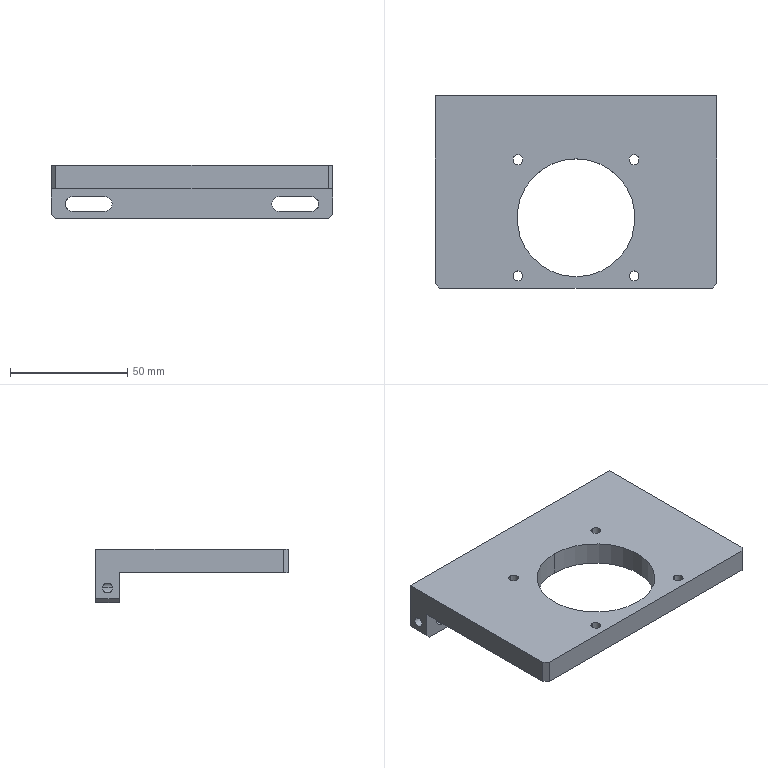Part | 1 solid | 36 faces | box 120 x 82 x 22.8 mm | volume 90820 mm3 | cylinder 20 | plane 16 | commonest cylinder face diameters 4.2 x12 6.3 x6 50.2 x2
STEP:
#1=CARTESIAN_POINT('',(-24.749,-37.849,0.));
#2=VERTEX_POINT('',#1);
#3=CARTESIAN_POINT('',(-24.749,-33.649,0.));
#4=VERTEX_POINT('',#3);
#5=CARTESIAN_POINT('',(-24.749,-35.749,0.));
#6=DIRECTION('',(0.,0.,-1.));
#7=DIRECTION('',(0.,1.,0.));
#8=AXIS2_PLACEMENT_3D('',#5,#6,#7);
#9=CIRCLE('',#8,2.1);
#10=EDGE_CURVE('',#2,#4,#9,.T.);
#11=ORIENTED_EDGE('',*,*,#10,.F.);
#12=CARTESIAN_POINT('',(-24.749,-37.849,-10.));
#13=VERTEX_POINT('',#12);
#14=CARTESIAN_POINT('',(-24.749,-37.849,-10.));
#15=DIRECTION('',(0.,0.,-1.));
#16=VECTOR('',#15,1000.);
#17=LINE('',#14,#16);
#18=EDGE_CURVE('',#13,#2,#17,.F.);
#19=ORIENTED_EDGE('',*,*,#18,.F.);
#20=CARTESIAN_POINT('',(-24.749,-33.649,-10.));
#21=VERTEX_POINT('',#20);
#22=CARTESIAN_POINT('',(-24.749,-35.749,-10.));
#23=DIRECTION('',(0.,0.,-1.));
#24=DIRECTION('',(0.,1.,0.));
#25=AXIS2_PLACEMENT_3D('',#22,#23,#24);
#26=CIRCLE('',#25,2.1);
#27=EDGE_CURVE('',#13,#21,#26,.T.);
#28=ORIENTED_EDGE('',*,*,#27,.T.);
#29=CARTESIAN_POINT('',(-24.749,-33.649,-10.));
#30=DIRECTION('',(0.,0.,-1.));
#31=VECTOR('',#30,1000.);
#32=LINE('',#29,#31);
#33=EDGE_CURVE('',#21,#4,#32,.F.);
#34=ORIENTED_EDGE('',*,*,#33,.T.);
#35=EDGE_LOOP('',(#11,#19,#28,#34));
#36=FACE_BOUND('',#35,.T.);
#37=CARTESIAN_POINT('',(-24.749,-35.749,-10.));
#38=DIRECTION('',(0.,0.,-1.));
#39=DIRECTION('',(0.,-1.,0.));
#40=AXIS2_PLACEMENT_3D('',#37,#38,#39);
#41=CYLINDRICAL_SURFACE('',#40,2.1);
#42=ADVANCED_FACE('',(#36),#41,.F.);
#43=CARTESIAN_POINT('',(24.749,-37.849,0.));
#44=VERTEX_POINT('',#43);
#45=CARTESIAN_POINT('',(24.749,-33.649,0.));
#46=VERTEX_POINT('',#45);
#47=CARTESIAN_POINT('',(24.749,-35.749,0.));
#48=DIRECTION('',(0.,0.,-1.));
#49=DIRECTION('',(0.,1.,0.));
#50=AXIS2_PLACEMENT_3D('',#47,#48,#49);
#51=CIRCLE('',#50,2.1);
#52=EDGE_CURVE('',#44,#46,#51,.T.);
#53=ORIENTED_EDGE('',*,*,#52,.F.);
#54=CARTESIAN_POINT('',(24.749,-37.849,-10.));
#55=VERTEX_POINT('',#54);
#56=CARTESIAN_POINT('',(24.749,-37.849,-10.));
#57=DIRECTION('',(0.,0.,-1.));
#58=VECTOR('',#57,1000.);
#59=LINE('',#56,#58);
#60=EDGE_CURVE('',#55,#44,#59,.F.);
#61=ORIENTED_EDGE('',*,*,#60,.F.);
#62=CARTESIAN_POINT('',(24.749,-33.649,-10.));
#63=VERTEX_POINT('',#62);
#64=CARTESIAN_POINT('',(24.749,-35.749,-10.));
#65=DIRECTION('',(0.,0.,-1.));
#66=DIRECTION('',(0.,1.,0.));
#67=AXIS2_PLACEMENT_3D('',#64,#65,#66);
#68=CIRCLE('',#67,2.1);
#69=EDGE_CURVE('',#55,#63,#68,.T.);
#70=ORIENTED_EDGE('',*,*,#69,.T.);
#71=CARTESIAN_POINT('',(24.749,-33.649,-10.));
#72=DIRECTION('',(0.,0.,-1.));
#73=VECTOR('',#72,1000.);
#74=LINE('',#71,#73);
#75=EDGE_CURVE('',#63,#46,#74,.F.);
#76=ORIENTED_EDGE('',*,*,#75,.T.);
#77=EDGE_LOOP('',(#53,#61,#70,#76));
#78=FACE_BOUND('',#77,.T.);
#79=CARTESIAN_POINT('',(24.749,-35.749,-10.));
#80=DIRECTION('',(0.,0.,-1.));
#81=DIRECTION('',(0.,-1.,0.));
#82=AXIS2_PLACEMENT_3D('',#79,#80,#81);
#83=CYLINDRICAL_SURFACE('',#82,2.1);
#84=ADVANCED_FACE('',(#78),#83,.F.);
#85=CARTESIAN_POINT('',(-24.749,11.649,0.));
#86=VERTEX_POINT('',#85);
#87=CARTESIAN_POINT('',(-24.749,15.849,0.));
#88=VERTEX_POINT('',#87);
#89=CARTESIAN_POINT('',(-24.749,13.749,0.));
#90=DIRECTION('',(0.,0.,-1.));
#91=DIRECTION('',(0.,1.,0.));
#92=AXIS2_PLACEMENT_3D('',#89,#90,#91);
#93=CIRCLE('',#92,2.1);
#94=EDGE_CURVE('',#86,#88,#93,.T.);
#95=ORIENTED_EDGE('',*,*,#94,.F.);
#96=CARTESIAN_POINT('',(-24.749,11.649,-10.));
#97=VERTEX_POINT('',#96);
#98=CARTESIAN_POINT('',(-24.749,11.649,-10.));
#99=DIRECTION('',(0.,0.,-1.));
#100=VECTOR('',#99,1000.);
#101=LINE('',#98,#100);
#102=EDGE_CURVE('',#97,#86,#101,.F.);
#103=ORIENTED_EDGE('',*,*,#102,.F.);
#104=CARTESIAN_POINT('',(-24.749,15.849,-10.));
#105=VERTEX_POINT('',#104);
#106=CARTESIAN_POINT('',(-24.749,13.749,-10.));
#107=DIRECTION('',(0.,0.,-1.));
#108=DIRECTION('',(0.,1.,0.));
#109=AXIS2_PLACEMENT_3D('',#106,#107,#108);
#110=CIRCLE('',#109,2.1);
#111=EDGE_CURVE('',#97,#105,#110,.T.);
#112=ORIENTED_EDGE('',*,*,#111,.T.);
#113=CARTESIAN_POINT('',(-24.749,15.849,-10.));
#114=DIRECTION('',(0.,0.,-1.));
#115=VECTOR('',#114,1000.);
#116=LINE('',#113,#115);
#117=EDGE_CURVE('',#105,#88,#116,.F.);
#118=ORIENTED_EDGE('',*,*,#117,.T.);
#119=EDGE_LOOP('',(#95,#103,#112,#118));
#120=FACE_BOUND('',#119,.T.);
#121=CARTESIAN_POINT('',(-24.749,13.749,-10.));
#122=DIRECTION('',(0.,0.,-1.));
#123=DIRECTION('',(0.,-1.,0.));
#124=AXIS2_PLACEMENT_3D('',#121,#122,#123);
#125=CYLINDRICAL_SURFACE('',#124,2.1);
#126=ADVANCED_FACE('',(#120),#125,.F.);
#127=CARTESIAN_POINT('',(24.749,11.649,0.));
#128=VERTEX_POINT('',#127);
#129=CARTESIAN_POINT('',(24.749,15.849,0.));
#130=VERTEX_POINT('',#129);
#131=CARTESIAN_POINT('',(24.749,13.749,0.));
#132=DIRECTION('',(0.,0.,-1.));
#133=DIRECTION('',(0.,1.,0.));
#134=AXIS2_PLACEMENT_3D('',#131,#132,#133);
#135=CIRCLE('',#134,2.1);
#136=EDGE_CURVE('',#128,#130,#135,.T.);
#137=ORIENTED_EDGE('',*,*,#136,.F.);
#138=CARTESIAN_POINT('',(24.749,11.649,-10.));
#139=VERTEX_POINT('',#138);
#140=CARTESIAN_POINT('',(24.749,11.649,-10.));
#141=DIRECTION('',(0.,0.,-1.));
#142=VECTOR('',#141,1000.);
#143=LINE('',#140,#142);
#144=EDGE_CURVE('',#139,#128,#143,.F.);
#145=ORIENTED_EDGE('',*,*,#144,.F.);
#146=CARTESIAN_POINT('',(24.749,15.849,-10.));
#147=VERTEX_POINT('',#146);
#148=CARTESIAN_POINT('',(24.749,13.749,-10.));
#149=DIRECTION('',(0.,0.,-1.));
#150=DIRECTION('',(0.,1.,0.));
#151=AXIS2_PLACEMENT_3D('',#148,#149,#150);
#152=CIRCLE('',#151,2.1);
#153=EDGE_CURVE('',#139,#147,#152,.T.);
#154=ORIENTED_EDGE('',*,*,#153,.T.);
#155=CARTESIAN_POINT('',(24.749,15.849,-10.));
#156=DIRECTION('',(0.,0.,-1.));
#157=VECTOR('',#156,1000.);
#158=LINE('',#155,#157);
#159=EDGE_CURVE('',#147,#130,#158,.F.);
#160=ORIENTED_EDGE('',*,*,#159,.T.);
#161=EDGE_LOOP('',(#137,#145,#154,#160));
#162=FACE_BOUND('',#161,.T.);
#163=CARTESIAN_POINT('',(24.749,13.749,-10.));
#164=DIRECTION('',(0.,0.,-1.));
#165=DIRECTION('',(0.,-1.,0.));
#166=AXIS2_PLACEMENT_3D('',#163,#164,#165);
#167=CYLINDRICAL_SURFACE('',#166,2.1);
#168=ADVANCED_FACE('',(#162),#167,.F.);
#169=CARTESIAN_POINT('',(0.,14.1,-10.));
#170=VERTEX_POINT('',#169);
#171=CARTESIAN_POINT('',(0.,-36.1,-10.));
#172=VERTEX_POINT('',#171);
#173=CARTESIAN_POINT('',(0.,-11.,-10.));
#174=DIRECTION('',(0.,0.,1.));
#175=DIRECTION('',(-1.,0.,0.));
#176=AXIS2_PLACEMENT_3D('',#173,#174,#175);
#177=CIRCLE('',#176,25.1);
#178=EDGE_CURVE('',#170,#172,#177,.T.);
#179=ORIENTED_EDGE('',*,*,#178,.F.);
#180=CARTESIAN_POINT('',(0.,14.1,0.));
#181=VERTEX_POINT('',#180);
#182=CARTESIAN_POINT('',(0.,14.1,0.));
#183=DIRECTION('',(0.,0.,1.));
#184=VECTOR('',#183,1000.);
#185=LINE('',#182,#184);
#186=EDGE_CURVE('',#181,#170,#185,.F.);
#187=ORIENTED_EDGE('',*,*,#186,.F.);
#188=CARTESIAN_POINT('',(0.,-36.1,0.));
#189=VERTEX_POINT('',#188);
#190=CARTESIAN_POINT('',(0.,-11.,0.));
#191=DIRECTION('',(0.,0.,1.));
#192=DIRECTION('',(0.,-1.,0.));
#193=AXIS2_PLACEMENT_3D('',#190,#191,#192);
#194=CIRCLE('',#193,25.1);
#195=EDGE_CURVE('',#181,#189,#194,.T.);
#196=ORIENTED_EDGE('',*,*,#195,.T.);
#197=CARTESIAN_POINT('',(0.,-36.1,0.));
#198=DIRECTION('',(0.,0.,1.));
#199=VECTOR('',#198,1000.);
#200=LINE('',#197,#199);
#201=EDGE_CURVE('',#189,#172,#200,.F.);
#202=ORIENTED_EDGE('',*,*,#201,.T.);
#203=EDGE_LOOP('',(#179,#187,#196,#202));
#204=FACE_BOUND('',#203,.T.);
#205=CARTESIAN_POINT('',(0.,-11.,0.));
#206=DIRECTION('',(0.,0.,1.));
#207=DIRECTION('',(0.,1.,0.));
#208=AXIS2_PLACEMENT_3D('',#205,#206,#207);
#209=CYLINDRICAL_SURFACE('',#208,25.1);
#210=ADVANCED_FACE('',(#204),#209,.F.);
#211=CARTESIAN_POINT('',(54.,33.9,-16.5));
#212=VERTEX_POINT('',#211);
#213=CARTESIAN_POINT('',(54.,38.1,-16.5));
#214=VERTEX_POINT('',#213);
#215=CARTESIAN_POINT('',(54.,33.9,-16.5));
#216=CARTESIAN_POINT('',(54.,33.9,-17.075));
#217=CARTESIAN_POINT('',(53.653,34.362,-18.14));
#218=CARTESIAN_POINT('',(52.971,35.995,-18.829));
#219=CARTESIAN_POINT('',(53.651,37.638,-18.143));
#220=CARTESIAN_POINT('',(54.,38.1,-17.075));
#221=CARTESIAN_POINT('',(54.,38.1,-16.5));
#222=B_SPLINE_CURVE_WITH_KNOTS('',3,(#215,#216,#217,#218,#219,#220,#221),.UNSPECIFIED.,.F.,.F.,(4,1,1,1,4),(0.,0.001696,0.003392,0.005088,0.006784),.UNSPECIFIED.);
#223=EDGE_CURVE('',#212,#214,#222,.T.);
#224=ORIENTED_EDGE('',*,*,#223,.F.);
#225=CARTESIAN_POINT('',(60.,33.9,-16.5));
#226=VERTEX_POINT('',#225);
#227=CARTESIAN_POINT('',(60.,33.9,-16.5));
#228=DIRECTION('',(1.,0.,0.));
#229=VECTOR('',#228,1000.);
#230=LINE('',#227,#229);
#231=EDGE_CURVE('',#226,#212,#230,.F.);
#232=ORIENTED_EDGE('',*,*,#231,.F.);
#233=CARTESIAN_POINT('',(60.,38.1,-16.5));
#234=VERTEX_POINT('',#233);
#235=CARTESIAN_POINT('',(60.,36.,-16.5));
#236=DIRECTION('',(1.,0.,0.));
#237=DIRECTION('',(0.,1.,0.));
#238=AXIS2_PLACEMENT_3D('',#235,#236,#237);
#239=CIRCLE('',#238,2.1);
#240=EDGE_CURVE('',#226,#234,#239,.T.);
#241=ORIENTED_EDGE('',*,*,#240,.T.);
#242=CARTESIAN_POINT('',(60.,38.1,-16.5));
#243=DIRECTION('',(1.,0.,0.));
#244=VECTOR('',#243,1000.);
#245=LINE('',#242,#244);
#246=EDGE_CURVE('',#234,#214,#245,.F.);
#247=ORIENTED_EDGE('',*,*,#246,.T.);
#248=EDGE_LOOP('',(#224,#232,#241,#247));
#249=FACE_BOUND('',#248,.T.);
#250=CARTESIAN_POINT('',(60.,36.,-16.5));
#251=DIRECTION('',(1.,0.,0.));
#252=DIRECTION('',(0.,-1.,0.));
#253=AXIS2_PLACEMENT_3D('',#250,#251,#252);
#254=CYLINDRICAL_SURFACE('',#253,2.1);
#255=ADVANCED_FACE('',(#249),#254,.F.);
#256=CARTESIAN_POINT('',(-54.,38.1,-16.5));
#257=VERTEX_POINT('',#256);
#258=CARTESIAN_POINT('',(-54.,33.9,-16.5));
#259=VERTEX_POINT('',#258);
#260=CARTESIAN_POINT('',(-54.,38.1,-16.5));
#261=CARTESIAN_POINT('',(-54.,38.1,-17.075));
#262=CARTESIAN_POINT('',(-53.653,37.638,-18.14));
#263=CARTESIAN_POINT('',(-52.971,36.005,-18.829));
#264=CARTESIAN_POINT('',(-53.651,34.362,-18.143));
#265=CARTESIAN_POINT('',(-54.,33.9,-17.075));
#266=CARTESIAN_POINT('',(-54.,33.9,-16.5));
#267=B_SPLINE_CURVE_WITH_KNOTS('',3,(#260,#261,#262,#263,#264,#265,#266),.UNSPECIFIED.,.F.,.F.,(4,1,1,1,4),(0.,0.001696,0.003392,0.005088,0.006784),.UNSPECIFIED.);
#268=EDGE_CURVE('',#257,#259,#267,.T.);
#269=ORIENTED_EDGE('',*,*,#268,.F.);
#270=CARTESIAN_POINT('',(-60.,38.1,-16.5));
#271=VERTEX_POINT('',#270);
#272=CARTESIAN_POINT('',(-60.,38.1,-16.5));
#273=DIRECTION('',(-1.,0.,0.));
#274=VECTOR('',#273,1000.);
#275=LINE('',#272,#274);
#276=EDGE_CURVE('',#271,#257,#275,.F.);
#277=ORIENTED_EDGE('',*,*,#276,.F.);
#278=CARTESIAN_POINT('',(-60.,33.9,-16.5));
#279=VERTEX_POINT('',#278);
#280=CARTESIAN_POINT('',(-60.,36.,-16.5));
#281=DIRECTION('',(-1.,0.,0.));
#282=DIRECTION('',(0.,-1.,0.));
#283=AXIS2_PLACEMENT_3D('',#280,#281,#282);
#284=CIRCLE('',#283,2.1);
#285=EDGE_CURVE('',#271,#279,#284,.T.);
#286=ORIENTED_EDGE('',*,*,#285,.T.);
#287=CARTESIAN_POINT('',(-60.,33.9,-16.5));
#288=DIRECTION('',(-1.,0.,0.));
#289=VECTOR('',#288,1000.);
#290=LINE('',#287,#289);
#291=EDGE_CURVE('',#279,#259,#290,.F.);
#292=ORIENTED_EDGE('',*,*,#291,.T.);
#293=EDGE_LOOP('',(#269,#277,#286,#292));
#294=FACE_BOUND('',#293,.T.);
#295=CARTESIAN_POINT('',(-60.,36.,-16.5));
#296=DIRECTION('',(-1.,0.,0.));
#297=DIRECTION('',(0.,1.,0.));
#298=AXIS2_PLACEMENT_3D('',#295,#296,#297);
#299=CYLINDRICAL_SURFACE('',#298,2.1);
#300=ADVANCED_FACE('',(#294),#299,.F.);
#301=CARTESIAN_POINT('',(-34.,41.,-16.5));
#302=VERTEX_POINT('',#301);
#303=CARTESIAN_POINT('',(-37.15,41.,-13.35));
#304=VERTEX_POINT('',#303);
#305=CARTESIAN_POINT('',(-37.15,41.,-16.5));
#306=DIRECTION('',(0.,-1.,0.));
#307=DIRECTION('',(1.,0.,0.));
#308=AXIS2_PLACEMENT_3D('',#305,#306,#307);
#309=CIRCLE('',#308,3.15);
#310=EDGE_CURVE('',#302,#304,#309,.T.);
#311=ORIENTED_EDGE('',*,*,#310,.F.);
#312=CARTESIAN_POINT('',(-34.,31.,-16.5));
#313=VERTEX_POINT('',#312);
#314=CARTESIAN_POINT('',(-34.,31.,-16.5));
#315=DIRECTION('',(0.,-1.,0.));
#316=VECTOR('',#315,1000.);
#317=LINE('',#314,#316);
#318=EDGE_CURVE('',#302,#313,#317,.T.);
#319=ORIENTED_EDGE('',*,*,#318,.T.);
#320=CARTESIAN_POINT('',(-37.15,31.,-13.35));
#321=VERTEX_POINT('',#320);
#322=CARTESIAN_POINT('',(-37.15,31.,-16.5));
#323=DIRECTION('',(0.,-1.,0.));
#324=DIRECTION('',(1.,0.,0.));
#325=AXIS2_PLACEMENT_3D('',#322,#323,#324);
#326=CIRCLE('',#325,3.15);
#327=EDGE_CURVE('',#313,#321,#326,.T.);
#328=ORIENTED_EDGE('',*,*,#327,.T.);
#329=CARTESIAN_POINT('',(-37.15,31.,-13.35));
#330=DIRECTION('',(0.,-1.,0.));
#331=VECTOR('',#330,1000.);
#332=LINE('',#329,#331);
#333=EDGE_CURVE('',#304,#321,#332,.T.);
#334=ORIENTED_EDGE('',*,*,#333,.F.);
#335=EDGE_LOOP('',(#311,#319,#328,#334));
#336=FACE_BOUND('',#335,.T.);
#337=CARTESIAN_POINT('',(-37.15,31.,-16.5));
#338=DIRECTION('',(0.,-1.,0.));
#339=DIRECTION('',(-1.,0.,0.));
#340=AXIS2_PLACEMENT_3D('',#337,#338,#339);
#341=CYLINDRICAL_SURFACE('',#340,3.15);
#342=ADVANCED_FACE('',(#336),#341,.F.);
#343=CARTESIAN_POINT('',(54.,41.,-16.5));
#344=VERTEX_POINT('',#343);
#345=CARTESIAN_POINT('',(50.85,41.,-13.35));
#346=VERTEX_POINT('',#345);
#347=CARTESIAN_POINT('',(50.85,41.,-16.5));
#348=DIRECTION('',(0.,-1.,0.));
#349=DIRECTION('',(1.,0.,0.));
#350=AXIS2_PLACEMENT_3D('',#347,#348,#349);
#351=CIRCLE('',#350,3.15);
#352=EDGE_CURVE('',#344,#346,#351,.T.);
#353=ORIENTED_EDGE('',*,*,#352,.F.);
#354=CARTESIAN_POINT('',(54.,31.,-16.5));
#355=DIRECTION('',(0.,-1.,0.));
#356=VECTOR('',#355,1000.);
#357=LINE('',#354,#356);
#358=EDGE_CURVE('',#344,#214,#357,.T.);
#359=ORIENTED_EDGE('',*,*,#358,.T.);
#360=CARTESIAN_POINT('',(54.,38.1,-16.5));
#361=CARTESIAN_POINT('',(54.,38.1,-15.925));
#362=CARTESIAN_POINT('',(53.653,37.638,-14.86));
#363=CARTESIAN_POINT('',(52.971,36.005,-14.171));
#364=CARTESIAN_POINT('',(53.651,34.362,-14.857));
#365=CARTESIAN_POINT('',(54.,33.9,-15.925));
#366=CARTESIAN_POINT('',(54.,33.9,-16.5));
#367=B_SPLINE_CURVE_WITH_KNOTS('',3,(#360,#361,#362,#363,#364,#365,#366),.UNSPECIFIED.,.F.,.F.,(4,1,1,1,4),(0.,0.001696,0.003392,0.005088,0.006784),.UNSPECIFIED.);
#368=EDGE_CURVE('',#214,#212,#367,.T.);
#369=ORIENTED_EDGE('',*,*,#368,.T.);
#370=CARTESIAN_POINT('',(54.,31.,-16.5));
#371=VERTEX_POINT('',#370);
#372=CARTESIAN_POINT('',(54.,31.,-16.5));
#373=DIRECTION('',(0.,-1.,0.));
#374=VECTOR('',#373,1000.);
#375=LINE('',#372,#374);
#376=EDGE_CURVE('',#212,#371,#375,.T.);
#377=ORIENTED_EDGE('',*,*,#376,.T.);
#378=CARTESIAN_POINT('',(50.85,31.,-13.35));
#379=VERTEX_POINT('',#378);
#380=CARTESIAN_POINT('',(50.85,31.,-16.5));
#381=DIRECTION('',(0.,-1.,0.));
#382=DIRECTION('',(1.,0.,0.));
#383=AXIS2_PLACEMENT_3D('',#380,#381,#382);
#384=CIRCLE('',#383,3.15);
#385=EDGE_CURVE('',#371,#379,#384,.T.);
#386=ORIENTED_EDGE('',*,*,#385,.T.);
#387=CARTESIAN_POINT('',(50.85,31.,-13.35));
#388=DIRECTION('',(0.,-1.,0.));
#389=VECTOR('',#388,1000.);
#390=LINE('',#387,#389);
#391=EDGE_CURVE('',#346,#379,#390,.T.);
#392=ORIENTED_EDGE('',*,*,#391,.F.);
#393=EDGE_LOOP('',(#353,#359,#369,#377,#386,#392));
#394=FACE_BOUND('',#393,.T.);
#395=CARTESIAN_POINT('',(50.85,31.,-16.5));
#396=DIRECTION('',(0.,-1.,0.));
#397=DIRECTION('',(-1.,0.,0.));
#398=AXIS2_PLACEMENT_3D('',#395,#396,#397);
#399=CYLINDRICAL_SURFACE('',#398,3.15);
#400=ADVANCED_FACE('',(#394),#399,.F.);
#401=CARTESIAN_POINT('',(-50.85,41.,-13.35));
#402=VERTEX_POINT('',#401);
#403=CARTESIAN_POINT('',(-50.85,41.,-19.65));
#404=VERTEX_POINT('',#403);
#405=CARTESIAN_POINT('',(-50.85,41.,-16.5));
#406=DIRECTION('',(0.,-1.,0.));
#407=DIRECTION('',(1.,0.,0.));
#408=AXIS2_PLACEMENT_3D('',#405,#406,#407);
#409=CIRCLE('',#408,3.15);
#410=EDGE_CURVE('',#402,#404,#409,.T.);
#411=ORIENTED_EDGE('',*,*,#410,.T.);
#412=CARTESIAN_POINT('',(-37.15,41.,-19.65));
#413=VERTEX_POINT('',#412);
#414=CARTESIAN_POINT('',(-50.85,41.,-19.65));
#415=DIRECTION('',(1.,0.,0.));
#416=VECTOR('',#415,1000.);
#417=LINE('',#414,#416);
#418=EDGE_CURVE('',#404,#413,#417,.T.);
#419=ORIENTED_EDGE('',*,*,#418,.T.);
#420=CARTESIAN_POINT('',(-37.15,41.,-16.5));
#421=DIRECTION('',(0.,-1.,0.));
#422=DIRECTION('',(1.,0.,0.));
#423=AXIS2_PLACEMENT_3D('',#420,#421,#422);
#424=CIRCLE('',#423,3.15);
#425=EDGE_CURVE('',#413,#302,#424,.T.);
#426=ORIENTED_EDGE('',*,*,#425,.T.);
#427=ORIENTED_EDGE('',*,*,#310,.T.);
#428=CARTESIAN_POINT('',(-50.85,41.,-13.35));
#429=DIRECTION('',(1.,0.,0.));
#430=VECTOR('',#429,1000.);
#431=LINE('',#428,#430);
#432=EDGE_CURVE('',#402,#304,#431,.T.);
#433=ORIENTED_EDGE('',*,*,#432,.F.);
#434=EDGE_LOOP('',(#411,#419,#426,#427,#433));
#435=FACE_BOUND('',#434,.T.);
#436=CARTESIAN_POINT('',(-58.2,41.,-22.8));
#437=VERTEX_POINT('',#436);
#438=CARTESIAN_POINT('',(58.2,41.,-22.8));
#439=VERTEX_POINT('',#438);
#440=CARTESIAN_POINT('',(0.,41.,-22.8));
#441=DIRECTION('',(1.,0.,0.));
#442=VECTOR('',#441,1000.);
#443=LINE('',#440,#442);
#444=EDGE_CURVE('',#437,#439,#443,.T.);
#445=ORIENTED_EDGE('',*,*,#444,.F.);
#446=CARTESIAN_POINT('',(-60.,41.,-21.));
#447=VERTEX_POINT('',#446);
#448=CARTESIAN_POINT('',(-34.75,41.,-46.25));
#449=DIRECTION('',(-0.7071,0.,0.7071));
#450=VECTOR('',#449,1000.);
#451=LINE('',#448,#450);
#452=EDGE_CURVE('',#437,#447,#451,.T.);
#453=ORIENTED_EDGE('',*,*,#452,.T.);
#454=CARTESIAN_POINT('',(-60.,41.,0.));
#455=VERTEX_POINT('',#454);
#456=CARTESIAN_POINT('',(-60.,41.,0.));
#457=DIRECTION('',(0.,0.,-1.));
#458=VECTOR('',#457,1000.);
#459=LINE('',#456,#458);
#460=EDGE_CURVE('',#455,#447,#459,.T.);
#461=ORIENTED_EDGE('',*,*,#460,.F.);
#462=CARTESIAN_POINT('',(60.,41.,0.));
#463=VERTEX_POINT('',#462);
#464=CARTESIAN_POINT('',(60.,41.,0.));
#465=DIRECTION('',(-1.,0.,0.));
#466=VECTOR('',#465,1000.);
#467=LINE('',#464,#466);
#468=EDGE_CURVE('',#463,#455,#467,.T.);
#469=ORIENTED_EDGE('',*,*,#468,.F.);
#470=CARTESIAN_POINT('',(60.,41.,-21.));
#471=VERTEX_POINT('',#470);
#472=CARTESIAN_POINT('',(60.,41.,0.));
#473=DIRECTION('',(0.,0.,1.));
#474=VECTOR('',#473,1000.);
#475=LINE('',#472,#474);
#476=EDGE_CURVE('',#471,#463,#475,.T.);
#477=ORIENTED_EDGE('',*,*,#476,.F.);
#478=CARTESIAN_POINT('',(34.75,41.,-46.25));
#479=DIRECTION('',(-0.7071,0.,-0.7071));
#480=VECTOR('',#479,1000.);
#481=LINE('',#478,#480);
#482=EDGE_CURVE('',#471,#439,#481,.T.);
#483=ORIENTED_EDGE('',*,*,#482,.T.);
#484=EDGE_LOOP('',(#445,#453,#461,#469,#477,#483));
#485=FACE_BOUND('',#484,.T.);
#486=CARTESIAN_POINT('',(37.15,41.,-13.35));
#487=VERTEX_POINT('',#486);
#488=CARTESIAN_POINT('',(37.15,41.,-19.65));
#489=VERTEX_POINT('',#488);
#490=CARTESIAN_POINT('',(37.15,41.,-16.5));
#491=DIRECTION('',(0.,-1.,0.));
#492=DIRECTION('',(1.,0.,0.));
#493=AXIS2_PLACEMENT_3D('',#490,#491,#492);
#494=CIRCLE('',#493,3.15);
#495=EDGE_CURVE('',#487,#489,#494,.T.);
#496=ORIENTED_EDGE('',*,*,#495,.T.);
#497=CARTESIAN_POINT('',(50.85,41.,-19.65));
#498=VERTEX_POINT('',#497);
#499=CARTESIAN_POINT('',(37.15,41.,-19.65));
#500=DIRECTION('',(1.,0.,0.));
#501=VECTOR('',#500,1000.);
#502=LINE('',#499,#501);
#503=EDGE_CURVE('',#489,#498,#502,.T.);
#504=ORIENTED_EDGE('',*,*,#503,.T.);
#505=CARTESIAN_POINT('',(50.85,41.,-16.5));
#506=DIRECTION('',(0.,-1.,0.));
#507=DIRECTION('',(1.,0.,0.));
#508=AXIS2_PLACEMENT_3D('',#505,#506,#507);
#509=CIRCLE('',#508,3.15);
#510=EDGE_CURVE('',#498,#344,#509,.T.);
#511=ORIENTED_EDGE('',*,*,#510,.T.);
#512=ORIENTED_EDGE('',*,*,#352,.T.);
#513=CARTESIAN_POINT('',(37.15,41.,-13.35));
#514=DIRECTION('',(1.,0.,0.));
#515=VECTOR('',#514,1000.);
#516=LINE('',#513,#515);
#517=EDGE_CURVE('',#487,#346,#516,.T.);
#518=ORIENTED_EDGE('',*,*,#517,.F.);
#519=EDGE_LOOP('',(#496,#504,#511,#512,#518));
#520=FACE_BOUND('',#519,.T.);
#521=CARTESIAN_POINT('',(0.,41.,-11.5));
#522=DIRECTION('',(0.,1.,0.));
#523=DIRECTION('',(1.,0.,0.));
#524=AXIS2_PLACEMENT_3D('',#521,#522,#523);
#525=PLANE('',#524);
#526=ADVANCED_FACE('',(#435,#485,#520),#525,.T.);
#527=CARTESIAN_POINT('',(-50.85,31.,-19.65));
#528=VERTEX_POINT('',#527);
#529=CARTESIAN_POINT('',(-37.15,31.,-19.65));
#530=VERTEX_POINT('',#529);
#531=CARTESIAN_POINT('',(-50.85,31.,-19.65));
#532=DIRECTION('',(1.,0.,0.));
#533=VECTOR('',#532,1000.);
#534=LINE('',#531,#533);
#535=EDGE_CURVE('',#528,#530,#534,.T.);
#536=ORIENTED_EDGE('',*,*,#535,.F.);
#537=CARTESIAN_POINT('',(-50.85,31.,-13.35));
#538=VERTEX_POINT('',#537);
#539=CARTESIAN_POINT('',(-50.85,31.,-16.5));
#540=DIRECTION('',(0.,-1.,0.));
#541=DIRECTION('',(1.,0.,0.));
#542=AXIS2_PLACEMENT_3D('',#539,#540,#541);
#543=CIRCLE('',#542,3.15);
#544=EDGE_CURVE('',#538,#528,#543,.T.);
#545=ORIENTED_EDGE('',*,*,#544,.F.);
#546=CARTESIAN_POINT('',(-50.85,31.,-13.35));
#547=DIRECTION('',(1.,0.,0.));
#548=VECTOR('',#547,1000.);
#549=LINE('',#546,#548);
#550=EDGE_CURVE('',#538,#321,#549,.T.);
#551=ORIENTED_EDGE('',*,*,#550,.T.);
#552=ORIENTED_EDGE('',*,*,#327,.F.);
#553=CARTESIAN_POINT('',(-37.15,31.,-16.5));
#554=DIRECTION('',(0.,-1.,0.));
#555=DIRECTION('',(1.,0.,0.));
#556=AXIS2_PLACEMENT_3D('',#553,#554,#555);
#557=CIRCLE('',#556,3.15);
#558=EDGE_CURVE('',#530,#313,#557,.T.);
#559=ORIENTED_EDGE('',*,*,#558,.F.);
#560=EDGE_LOOP('',(#536,#545,#551,#552,#559));
#561=FACE_BOUND('',#560,.T.);
#562=CARTESIAN_POINT('',(-60.,31.,-10.));
#563=VERTEX_POINT('',#562);
#564=CARTESIAN_POINT('',(-60.,31.,-21.));
#565=VERTEX_POINT('',#564);
#566=CARTESIAN_POINT('',(-60.,31.,-23.));
#567=DIRECTION('',(0.,0.,-1.));
#568=VECTOR('',#567,1000.);
#569=LINE('',#566,#568);
#570=EDGE_CURVE('',#563,#565,#569,.T.);
#571=ORIENTED_EDGE('',*,*,#570,.T.);
#572=CARTESIAN_POINT('',(-58.2,31.,-22.8));
#573=VERTEX_POINT('',#572);
#574=CARTESIAN_POINT('',(-58.,31.,-23.));
#575=DIRECTION('',(0.7071,0.,-0.7071));
#576=VECTOR('',#575,1000.);
#577=LINE('',#574,#576);
#578=EDGE_CURVE('',#565,#573,#577,.T.);
#579=ORIENTED_EDGE('',*,*,#578,.T.);
#580=CARTESIAN_POINT('',(58.2,31.,-22.8));
#581=VERTEX_POINT('',#580);
#582=CARTESIAN_POINT('',(60.,31.,-22.8));
#583=DIRECTION('',(-1.,0.,0.));
#584=VECTOR('',#583,1000.);
#585=LINE('',#582,#584);
#586=EDGE_CURVE('',#581,#573,#585,.T.);
#587=ORIENTED_EDGE('',*,*,#586,.F.);
#588=CARTESIAN_POINT('',(60.,31.,-21.));
#589=VERTEX_POINT('',#588);
#590=CARTESIAN_POINT('',(60.,31.,-21.));
#591=DIRECTION('',(0.7071,0.,0.7071));
#592=VECTOR('',#591,1000.);
#593=LINE('',#590,#592);
#594=EDGE_CURVE('',#581,#589,#593,.T.);
#595=ORIENTED_EDGE('',*,*,#594,.T.);
#596=CARTESIAN_POINT('',(60.,31.,-10.));
#597=VERTEX_POINT('',#596);
#598=CARTESIAN_POINT('',(60.,31.,-23.));
#599=DIRECTION('',(0.,0.,-1.));
#600=VECTOR('',#599,1000.);
#601=LINE('',#598,#600);
#602=EDGE_CURVE('',#597,#589,#601,.T.);
#603=ORIENTED_EDGE('',*,*,#602,.F.);
#604=CARTESIAN_POINT('',(60.,31.,-10.));
#605=DIRECTION('',(-1.,0.,0.));
#606=VECTOR('',#605,1000.);
#607=LINE('',#604,#606);
#608=EDGE_CURVE('',#597,#563,#607,.T.);
#609=ORIENTED_EDGE('',*,*,#608,.T.);
#610=EDGE_LOOP('',(#571,#579,#587,#595,#603,#609));
#611=FACE_BOUND('',#610,.T.);
#612=CARTESIAN_POINT('',(50.85,31.,-19.65));
#613=VERTEX_POINT('',#612);
#614=CARTESIAN_POINT('',(50.85,31.,-16.5));
#615=DIRECTION('',(0.,-1.,0.));
#616=DIRECTION('',(1.,0.,0.));
#617=AXIS2_PLACEMENT_3D('',#614,#615,#616);
#618=CIRCLE('',#617,3.15);
#619=EDGE_CURVE('',#613,#371,#618,.T.);
#620=ORIENTED_EDGE('',*,*,#619,.F.);
#621=CARTESIAN_POINT('',(37.15,31.,-19.65));
#622=VERTEX_POINT('',#621);
#623=CARTESIAN_POINT('',(37.15,31.,-19.65));
#624=DIRECTION('',(1.,0.,0.));
#625=VECTOR('',#624,1000.);
#626=LINE('',#623,#625);
#627=EDGE_CURVE('',#622,#613,#626,.T.);
#628=ORIENTED_EDGE('',*,*,#627,.F.);
#629=CARTESIAN_POINT('',(37.15,31.,-13.35));
#630=VERTEX_POINT('',#629);
#631=CARTESIAN_POINT('',(37.15,31.,-16.5));
#632=DIRECTION('',(0.,-1.,0.));
#633=DIRECTION('',(1.,0.,0.));
#634=AXIS2_PLACEMENT_3D('',#631,#632,#633);
#635=CIRCLE('',#634,3.15);
#636=EDGE_CURVE('',#630,#622,#635,.T.);
#637=ORIENTED_EDGE('',*,*,#636,.F.);
#638=CARTESIAN_POINT('',(37.15,31.,-13.35));
#639=DIRECTION('',(1.,0.,0.));
#640=VECTOR('',#639,1000.);
#641=LINE('',#638,#640);
#642=EDGE_CURVE('',#630,#379,#641,.T.);
#643=ORIENTED_EDGE('',*,*,#642,.T.);
#644=ORIENTED_EDGE('',*,*,#385,.F.);
#645=EDGE_LOOP('',(#620,#628,#637,#643,#644));
#646=FACE_BOUND('',#645,.T.);
#647=CARTESIAN_POINT('',(60.,31.,-23.));
#648=DIRECTION('',(0.,1.,0.));
#649=DIRECTION('',(1.,0.,0.));
#650=AXIS2_PLACEMENT_3D('',#647,#648,#649);
#651=PLANE('',#650);
#652=ADVANCED_FACE('',(#561,#611,#646),#651,.F.);
#653=CARTESIAN_POINT('',(-60.,36.,-16.5));
#654=DIRECTION('',(-1.,0.,0.));
#655=DIRECTION('',(0.,-1.,0.));
#656=AXIS2_PLACEMENT_3D('',#653,#654,#655);
#657=CIRCLE('',#656,2.1);
#658=EDGE_CURVE('',#279,#271,#657,.T.);
#659=ORIENTED_EDGE('',*,*,#658,.F.);
#660=ORIENTED_EDGE('',*,*,#285,.F.);
#661=EDGE_LOOP('',(#659,#660));
#662=FACE_BOUND('',#661,.T.);
#663=ORIENTED_EDGE('',*,*,#460,.T.);
#664=CARTESIAN_POINT('',(-60.,-41.,-21.));
#665=DIRECTION('',(0.,-1.,0.));
#666=VECTOR('',#665,1000.);
#667=LINE('',#664,#666);
#668=EDGE_CURVE('',#447,#565,#667,.T.);
#669=ORIENTED_EDGE('',*,*,#668,.T.);
#670=ORIENTED_EDGE('',*,*,#570,.F.);
#671=CARTESIAN_POINT('',(-60.,-39.,-10.));
#672=VERTEX_POINT('',#671);
#673=CARTESIAN_POINT('',(-60.,-41.,-10.));
#674=DIRECTION('',(0.,1.,0.));
#675=VECTOR('',#674,1000.);
#676=LINE('',#673,#675);
#677=EDGE_CURVE('',#672,#563,#676,.T.);
#678=ORIENTED_EDGE('',*,*,#677,.F.);
#679=CARTESIAN_POINT('',(-60.,-39.,0.));
#680=VERTEX_POINT('',#679);
#681=CARTESIAN_POINT('',(-60.,-39.,0.));
#682=DIRECTION('',(0.,0.,1.));
#683=VECTOR('',#682,1000.);
#684=LINE('',#681,#683);
#685=EDGE_CURVE('',#672,#680,#684,.T.);
#686=ORIENTED_EDGE('',*,*,#685,.T.);
#687=CARTESIAN_POINT('',(-60.,-41.,0.));
#688=DIRECTION('',(0.,1.,0.));
#689=VECTOR('',#688,1000.);
#690=LINE('',#687,#689);
#691=EDGE_CURVE('',#680,#455,#690,.T.);
#692=ORIENTED_EDGE('',*,*,#691,.T.);
#693=EDGE_LOOP('',(#663,#669,#670,#678,#686,#692));
#694=FACE_BOUND('',#693,.T.);
#695=CARTESIAN_POINT('',(-60.,-41.,0.));
#696=DIRECTION('',(1.,0.,0.));
#697=DIRECTION('',(0.,-1.,0.));
#698=AXIS2_PLACEMENT_3D('',#695,#696,#697);
#699=PLANE('',#698);
#700=ADVANCED_FACE('',(#662,#694),#699,.F.);
#701=ORIENTED_EDGE('',*,*,#586,.T.);
#702=CARTESIAN_POINT('',(-58.2,-41.,-22.8));
#703=DIRECTION('',(0.,1.,0.));
#704=VECTOR('',#703,1000.);
#705=LINE('',#702,#704);
#706=EDGE_CURVE('',#573,#437,#705,.T.);
#707=ORIENTED_EDGE('',*,*,#706,.T.);
#708=ORIENTED_EDGE('',*,*,#444,.T.);
#709=CARTESIAN_POINT('',(58.2,-41.,-22.8));
#710=DIRECTION('',(0.,-1.,0.));
#711=VECTOR('',#710,1000.);
#712=LINE('',#709,#711);
#713=EDGE_CURVE('',#439,#581,#712,.T.);
#714=ORIENTED_EDGE('',*,*,#713,.T.);
#715=EDGE_LOOP('',(#701,#707,#708,#714));
#716=FACE_BOUND('',#715,.T.);
#717=CARTESIAN_POINT('',(60.,-41.,-22.8));
#718=DIRECTION('',(0.,0.,1.));
#719=DIRECTION('',(1.,0.,0.));
#720=AXIS2_PLACEMENT_3D('',#717,#718,#719);
#721=PLANE('',#720);
#722=ADVANCED_FACE('',(#716),#721,.F.);
#723=CARTESIAN_POINT('',(60.,36.,-16.5));
#724=DIRECTION('',(1.,0.,0.));
#725=DIRECTION('',(0.,1.,0.));
#726=AXIS2_PLACEMENT_3D('',#723,#724,#725);
#727=CIRCLE('',#726,2.1);
#728=EDGE_CURVE('',#234,#226,#727,.T.);
#729=ORIENTED_EDGE('',*,*,#728,.F.);
#730=ORIENTED_EDGE('',*,*,#240,.F.);
#731=EDGE_LOOP('',(#729,#730));
#732=FACE_BOUND('',#731,.T.);
#733=ORIENTED_EDGE('',*,*,#602,.T.);
#734=CARTESIAN_POINT('',(60.,-41.,-21.));
#735=DIRECTION('',(0.,1.,0.));
#736=VECTOR('',#735,1000.);
#737=LINE('',#734,#736);
#738=EDGE_CURVE('',#589,#471,#737,.T.);
#739=ORIENTED_EDGE('',*,*,#738,.T.);
#740=ORIENTED_EDGE('',*,*,#476,.T.);
#741=CARTESIAN_POINT('',(60.,-39.,0.));
#742=VERTEX_POINT('',#741);
#743=CARTESIAN_POINT('',(60.,-41.,0.));
#744=DIRECTION('',(0.,1.,0.));
#745=VECTOR('',#744,1000.);
#746=LINE('',#743,#745);
#747=EDGE_CURVE('',#742,#463,#746,.T.);
#748=ORIENTED_EDGE('',*,*,#747,.F.);
#749=CARTESIAN_POINT('',(60.,-39.,-10.));
#750=VERTEX_POINT('',#749);
#751=CARTESIAN_POINT('',(60.,-39.,0.));
#752=DIRECTION('',(0.,0.,-1.));
#753=VECTOR('',#752,1000.);
#754=LINE('',#751,#753);
#755=EDGE_CURVE('',#742,#750,#754,.T.);
#756=ORIENTED_EDGE('',*,*,#755,.T.);
#757=CARTESIAN_POINT('',(60.,-41.,-10.));
#758=DIRECTION('',(0.,1.,0.));
#759=VECTOR('',#758,1000.);
#760=LINE('',#757,#759);
#761=EDGE_CURVE('',#750,#597,#760,.T.);
#762=ORIENTED_EDGE('',*,*,#761,.T.);
#763=EDGE_LOOP('',(#733,#739,#740,#748,#756,#762));
#764=FACE_BOUND('',#763,.T.);
#765=CARTESIAN_POINT('',(60.,-41.,0.));
#766=DIRECTION('',(-1.,0.,0.));
#767=DIRECTION('',(0.,1.,0.));
#768=AXIS2_PLACEMENT_3D('',#765,#766,#767);
#769=PLANE('',#768);
#770=ADVANCED_FACE('',(#732,#764),#769,.F.);
#771=CARTESIAN_POINT('',(-24.749,-35.749,0.));
#772=DIRECTION('',(0.,0.,-1.));
#773=DIRECTION('',(0.,1.,0.));
#774=AXIS2_PLACEMENT_3D('',#771,#772,#773);
#775=CIRCLE('',#774,2.1);
#776=EDGE_CURVE('',#4,#2,#775,.T.);
#777=ORIENTED_EDGE('',*,*,#776,.T.);
#778=ORIENTED_EDGE('',*,*,#10,.T.);
#779=EDGE_LOOP('',(#777,#778));
#780=FACE_BOUND('',#779,.T.);
#781=CARTESIAN_POINT('',(24.749,-35.749,0.));
#782=DIRECTION('',(0.,0.,-1.));
#783=DIRECTION('',(0.,1.,0.));
#784=AXIS2_PLACEMENT_3D('',#781,#782,#783);
#785=CIRCLE('',#784,2.1);
#786=EDGE_CURVE('',#46,#44,#785,.T.);
#787=ORIENTED_EDGE('',*,*,#786,.T.);
#788=ORIENTED_EDGE('',*,*,#52,.T.);
#789=EDGE_LOOP('',(#787,#788));
#790=FACE_BOUND('',#789,.T.);
#791=CARTESIAN_POINT('',(-24.749,13.749,0.));
#792=DIRECTION('',(0.,0.,-1.));
#793=DIRECTION('',(0.,1.,0.));
#794=AXIS2_PLACEMENT_3D('',#791,#792,#793);
#795=CIRCLE('',#794,2.1);
#796=EDGE_CURVE('',#88,#86,#795,.T.);
#797=ORIENTED_EDGE('',*,*,#796,.T.);
#798=ORIENTED_EDGE('',*,*,#94,.T.);
#799=EDGE_LOOP('',(#797,#798));
#800=FACE_BOUND('',#799,.T.);
#801=CARTESIAN_POINT('',(24.749,13.749,0.));
#802=DIRECTION('',(0.,0.,-1.));
#803=DIRECTION('',(0.,1.,0.));
#804=AXIS2_PLACEMENT_3D('',#801,#802,#803);
#805=CIRCLE('',#804,2.1);
#806=EDGE_CURVE('',#130,#128,#805,.T.);
#807=ORIENTED_EDGE('',*,*,#806,.T.);
#808=ORIENTED_EDGE('',*,*,#136,.T.);
#809=EDGE_LOOP('',(#807,#808));
#810=FACE_BOUND('',#809,.T.);
#811=CARTESIAN_POINT('',(0.,-11.,0.));
#812=DIRECTION('',(0.,0.,1.));
#813=DIRECTION('',(0.,-1.,0.));
#814=AXIS2_PLACEMENT_3D('',#811,#812,#813);
#815=CIRCLE('',#814,25.1);
#816=EDGE_CURVE('',#189,#181,#815,.T.);
#817=ORIENTED_EDGE('',*,*,#816,.F.);
#818=ORIENTED_EDGE('',*,*,#195,.F.);
#819=EDGE_LOOP('',(#817,#818));
#820=FACE_BOUND('',#819,.T.);
#821=ORIENTED_EDGE('',*,*,#691,.F.);
#822=CARTESIAN_POINT('',(-58.,-41.,0.));
#823=VERTEX_POINT('',#822);
#824=CARTESIAN_POINT('',(-58.,-41.,0.));
#825=DIRECTION('',(0.7071,-0.7071,0.));
#826=VECTOR('',#825,1000.);
#827=LINE('',#824,#826);
#828=EDGE_CURVE('',#680,#823,#827,.T.);
#829=ORIENTED_EDGE('',*,*,#828,.T.);
#830=CARTESIAN_POINT('',(58.,-41.,0.));
#831=VERTEX_POINT('',#830);
#832=CARTESIAN_POINT('',(60.,-41.,0.));
#833=DIRECTION('',(-1.,0.,0.));
#834=VECTOR('',#833,1000.);
#835=LINE('',#832,#834);
#836=EDGE_CURVE('',#831,#823,#835,.T.);
#837=ORIENTED_EDGE('',*,*,#836,.F.);
#838=CARTESIAN_POINT('',(58.,-41.,0.));
#839=DIRECTION('',(0.7071,0.7071,0.));
#840=VECTOR('',#839,1000.);
#841=LINE('',#838,#840);
#842=EDGE_CURVE('',#831,#742,#841,.T.);
#843=ORIENTED_EDGE('',*,*,#842,.T.);
#844=ORIENTED_EDGE('',*,*,#747,.T.);
#845=ORIENTED_EDGE('',*,*,#468,.T.);
#846=EDGE_LOOP('',(#821,#829,#837,#843,#844,#845));
#847=FACE_BOUND('',#846,.T.);
#848=CARTESIAN_POINT('',(60.,-41.,0.));
#849=DIRECTION('',(0.,0.,-1.));
#850=DIRECTION('',(-1.,0.,0.));
#851=AXIS2_PLACEMENT_3D('',#848,#849,#850);
#852=PLANE('',#851);
#853=ADVANCED_FACE('',(#780,#790,#800,#810,#820,#847),#852,.F.);
#854=ORIENTED_EDGE('',*,*,#836,.T.);
#855=CARTESIAN_POINT('',(-58.,-41.,-10.));
#856=VERTEX_POINT('',#855);
#857=CARTESIAN_POINT('',(-58.,-41.,-11.5));
#858=DIRECTION('',(0.,0.,-1.));
#859=VECTOR('',#858,1000.);
#860=LINE('',#857,#859);
#861=EDGE_CURVE('',#823,#856,#860,.T.);
#862=ORIENTED_EDGE('',*,*,#861,.T.);
#863=CARTESIAN_POINT('',(58.,-41.,-10.));
#864=VERTEX_POINT('',#863);
#865=CARTESIAN_POINT('',(60.,-41.,-10.));
#866=DIRECTION('',(-1.,0.,0.));
#867=VECTOR('',#866,1000.);
#868=LINE('',#865,#867);
#869=EDGE_CURVE('',#864,#856,#868,.T.);
#870=ORIENTED_EDGE('',*,*,#869,.F.);
#871=CARTESIAN_POINT('',(58.,-41.,-11.5));
#872=DIRECTION('',(0.,0.,1.));
#873=VECTOR('',#872,1000.);
#874=LINE('',#871,#873);
#875=EDGE_CURVE('',#864,#831,#874,.T.);
#876=ORIENTED_EDGE('',*,*,#875,.T.);
#877=EDGE_LOOP('',(#854,#862,#870,#876));
#878=FACE_BOUND('',#877,.T.);
#879=CARTESIAN_POINT('',(0.,-41.,-11.5));
#880=DIRECTION('',(0.,1.,0.));
#881=DIRECTION('',(1.,0.,0.));
#882=AXIS2_PLACEMENT_3D('',#879,#880,#881);
#883=PLANE('',#882);
#884=ADVANCED_FACE('',(#878),#883,.F.);
#885=CARTESIAN_POINT('',(-24.749,-35.749,-10.));
#886=DIRECTION('',(0.,0.,-1.));
#887=DIRECTION('',(0.,1.,0.));
#888=AXIS2_PLACEMENT_3D('',#885,#886,#887);
#889=CIRCLE('',#888,2.1);
#890=EDGE_CURVE('',#21,#13,#889,.T.);
#891=ORIENTED_EDGE('',*,*,#890,.F.);
#892=ORIENTED_EDGE('',*,*,#27,.F.);
#893=EDGE_LOOP('',(#891,#892));
#894=FACE_BOUND('',#893,.T.);
#895=CARTESIAN_POINT('',(24.749,-35.749,-10.));
#896=DIRECTION('',(0.,0.,-1.));
#897=DIRECTION('',(0.,1.,0.));
#898=AXIS2_PLACEMENT_3D('',#895,#896,#897);
#899=CIRCLE('',#898,2.1);
#900=EDGE_CURVE('',#63,#55,#899,.T.);
#901=ORIENTED_EDGE('',*,*,#900,.F.);
#902=ORIENTED_EDGE('',*,*,#69,.F.);
#903=EDGE_LOOP('',(#901,#902));
#904=FACE_BOUND('',#903,.T.);
#905=CARTESIAN_POINT('',(-24.749,13.749,-10.));
#906=DIRECTION('',(0.,0.,-1.));
#907=DIRECTION('',(0.,1.,0.));
#908=AXIS2_PLACEMENT_3D('',#905,#906,#907);
#909=CIRCLE('',#908,2.1);
#910=EDGE_CURVE('',#105,#97,#909,.T.);
#911=ORIENTED_EDGE('',*,*,#910,.F.);
#912=ORIENTED_EDGE('',*,*,#111,.F.);
#913=EDGE_LOOP('',(#911,#912));
#914=FACE_BOUND('',#913,.T.);
#915=CARTESIAN_POINT('',(24.749,13.749,-10.));
#916=DIRECTION('',(0.,0.,-1.));
#917=DIRECTION('',(0.,1.,0.));
#918=AXIS2_PLACEMENT_3D('',#915,#916,#917);
#919=CIRCLE('',#918,2.1);
#920=EDGE_CURVE('',#147,#139,#919,.T.);
#921=ORIENTED_EDGE('',*,*,#920,.F.);
#922=ORIENTED_EDGE('',*,*,#153,.F.);
#923=EDGE_LOOP('',(#921,#922));
#924=FACE_BOUND('',#923,.T.);
#925=CARTESIAN_POINT('',(0.,-11.,-10.));
#926=DIRECTION('',(0.,0.,1.));
#927=DIRECTION('',(-1.,0.,0.));
#928=AXIS2_PLACEMENT_3D('',#925,#926,#927);
#929=CIRCLE('',#928,25.1);
#930=EDGE_CURVE('',#172,#170,#929,.T.);
#931=ORIENTED_EDGE('',*,*,#930,.T.);
#932=ORIENTED_EDGE('',*,*,#178,.T.);
#933=EDGE_LOOP('',(#931,#932));
#934=FACE_BOUND('',#933,.T.);
#935=ORIENTED_EDGE('',*,*,#869,.T.);
#936=CARTESIAN_POINT('',(-58.,-41.,-10.));
#937=DIRECTION('',(-0.7071,0.7071,0.));
#938=VECTOR('',#937,1000.);
#939=LINE('',#936,#938);
#940=EDGE_CURVE('',#856,#672,#939,.T.);
#941=ORIENTED_EDGE('',*,*,#940,.T.);
#942=ORIENTED_EDGE('',*,*,#677,.T.);
#943=ORIENTED_EDGE('',*,*,#608,.F.);
#944=ORIENTED_EDGE('',*,*,#761,.F.);
#945=CARTESIAN_POINT('',(58.,-41.,-10.));
#946=DIRECTION('',(-0.7071,-0.7071,0.));
#947=VECTOR('',#946,1000.);
#948=LINE('',#945,#947);
#949=EDGE_CURVE('',#750,#864,#948,.T.);
#950=ORIENTED_EDGE('',*,*,#949,.T.);
#951=EDGE_LOOP('',(#935,#941,#942,#943,#944,#950));
#952=FACE_BOUND('',#951,.T.);
#953=CARTESIAN_POINT('',(60.,-41.,-10.));
#954=DIRECTION('',(0.,0.,1.));
#955=DIRECTION('',(1.,0.,0.));
#956=AXIS2_PLACEMENT_3D('',#953,#954,#955);
#957=PLANE('',#956);
#958=ADVANCED_FACE('',(#894,#904,#914,#924,#934,#952),#957,.F.);
#959=ORIENTED_EDGE('',*,*,#358,.F.);
#960=ORIENTED_EDGE('',*,*,#510,.F.);
#961=CARTESIAN_POINT('',(50.85,31.,-19.65));
#962=DIRECTION('',(0.,1.,0.));
#963=VECTOR('',#962,1000.);
#964=LINE('',#961,#963);
#965=EDGE_CURVE('',#613,#498,#964,.T.);
#966=ORIENTED_EDGE('',*,*,#965,.F.);
#967=ORIENTED_EDGE('',*,*,#619,.T.);
#968=ORIENTED_EDGE('',*,*,#376,.F.);
#969=ORIENTED_EDGE('',*,*,#223,.T.);
#970=EDGE_LOOP('',(#959,#960,#966,#967,#968,#969));
#971=FACE_BOUND('',#970,.T.);
#972=CARTESIAN_POINT('',(50.85,31.,-16.5));
#973=DIRECTION('',(0.,-1.,0.));
#974=DIRECTION('',(-1.,0.,0.));
#975=AXIS2_PLACEMENT_3D('',#972,#973,#974);
#976=CYLINDRICAL_SURFACE('',#975,3.15);
#977=ADVANCED_FACE('',(#971),#976,.F.);
#978=ORIENTED_EDGE('',*,*,#636,.T.);
#979=CARTESIAN_POINT('',(37.15,31.,-19.65));
#980=DIRECTION('',(0.,-1.,0.));
#981=VECTOR('',#980,1000.);
#982=LINE('',#979,#981);
#983=EDGE_CURVE('',#489,#622,#982,.T.);
#984=ORIENTED_EDGE('',*,*,#983,.F.);
#985=ORIENTED_EDGE('',*,*,#495,.F.);
#986=CARTESIAN_POINT('',(37.15,31.,-13.35));
#987=DIRECTION('',(0.,1.,0.));
#988=VECTOR('',#987,1000.);
#989=LINE('',#986,#988);
#990=EDGE_CURVE('',#630,#487,#989,.T.);
#991=ORIENTED_EDGE('',*,*,#990,.F.);
#992=EDGE_LOOP('',(#978,#984,#985,#991));
#993=FACE_BOUND('',#992,.T.);
#994=CARTESIAN_POINT('',(37.15,31.,-16.5));
#995=DIRECTION('',(0.,-1.,0.));
#996=DIRECTION('',(-1.,0.,0.));
#997=AXIS2_PLACEMENT_3D('',#994,#995,#996);
#998=CYLINDRICAL_SURFACE('',#997,3.15);
#999=ADVANCED_FACE('',(#993),#998,.F.);
#1000=ORIENTED_EDGE('',*,*,#391,.T.);
#1001=ORIENTED_EDGE('',*,*,#642,.F.);
#1002=ORIENTED_EDGE('',*,*,#990,.T.);
#1003=ORIENTED_EDGE('',*,*,#517,.T.);
#1004=EDGE_LOOP('',(#1000,#1001,#1002,#1003));
#1005=FACE_BOUND('',#1004,.T.);
#1006=CARTESIAN_POINT('',(37.15,31.,-13.35));
#1007=DIRECTION('',(0.,0.,1.));
#1008=DIRECTION('',(1.,0.,0.));
#1009=AXIS2_PLACEMENT_3D('',#1006,#1007,#1008);
#1010=PLANE('',#1009);
#1011=ADVANCED_FACE('',(#1005),#1010,.F.);
#1012=ORIENTED_EDGE('',*,*,#965,.T.);
#1013=ORIENTED_EDGE('',*,*,#503,.F.);
#1014=ORIENTED_EDGE('',*,*,#983,.T.);
#1015=ORIENTED_EDGE('',*,*,#627,.T.);
#1016=EDGE_LOOP('',(#1012,#1013,#1014,#1015));
#1017=FACE_BOUND('',#1016,.T.);
#1018=CARTESIAN_POINT('',(37.15,31.,-19.65));
#1019=DIRECTION('',(0.,0.,-1.));
#1020=DIRECTION('',(-1.,0.,0.));
#1021=AXIS2_PLACEMENT_3D('',#1018,#1019,#1020);
#1022=PLANE('',#1021);
#1023=ADVANCED_FACE('',(#1017),#1022,.F.);
#1024=ORIENTED_EDGE('',*,*,#318,.F.);
#1025=ORIENTED_EDGE('',*,*,#425,.F.);
#1026=CARTESIAN_POINT('',(-37.15,31.,-19.65));
#1027=DIRECTION('',(0.,1.,0.));
#1028=VECTOR('',#1027,1000.);
#1029=LINE('',#1026,#1028);
#1030=EDGE_CURVE('',#530,#413,#1029,.T.);
#1031=ORIENTED_EDGE('',*,*,#1030,.F.);
#1032=ORIENTED_EDGE('',*,*,#558,.T.);
#1033=EDGE_LOOP('',(#1024,#1025,#1031,#1032));
#1034=FACE_BOUND('',#1033,.T.);
#1035=CARTESIAN_POINT('',(-37.15,31.,-16.5));
#1036=DIRECTION('',(0.,-1.,0.));
#1037=DIRECTION('',(-1.,0.,0.));
#1038=AXIS2_PLACEMENT_3D('',#1035,#1036,#1037);
#1039=CYLINDRICAL_SURFACE('',#1038,3.15);
#1040=ADVANCED_FACE('',(#1034),#1039,.F.);
#1041=CARTESIAN_POINT('',(-54.,33.9,-16.5));
#1042=CARTESIAN_POINT('',(-54.,33.9,-15.925));
#1043=CARTESIAN_POINT('',(-53.653,34.362,-14.86));
#1044=CARTESIAN_POINT('',(-52.971,35.995,-14.171));
#1045=CARTESIAN_POINT('',(-53.651,37.638,-14.857));
#1046=CARTESIAN_POINT('',(-54.,38.1,-15.925));
#1047=CARTESIAN_POINT('',(-54.,38.1,-16.5));
#1048=B_SPLINE_CURVE_WITH_KNOTS('',3,(#1041,#1042,#1043,#1044,#1045,#1046,#1047),.UNSPECIFIED.,.F.,.F.,(4,1,1,1,4),(0.,0.001696,0.003392,0.005088,0.006784),.UNSPECIFIED.);
#1049=EDGE_CURVE('',#259,#257,#1048,.T.);
#1050=ORIENTED_EDGE('',*,*,#1049,.T.);
#1051=ORIENTED_EDGE('',*,*,#268,.T.);
#1052=EDGE_LOOP('',(#1050,#1051));
#1053=FACE_BOUND('',#1052,.T.);
#1054=ORIENTED_EDGE('',*,*,#544,.T.);
#1055=CARTESIAN_POINT('',(-50.85,31.,-19.65));
#1056=DIRECTION('',(0.,-1.,0.));
#1057=VECTOR('',#1056,1000.);
#1058=LINE('',#1055,#1057);
#1059=EDGE_CURVE('',#404,#528,#1058,.T.);
#1060=ORIENTED_EDGE('',*,*,#1059,.F.);
#1061=ORIENTED_EDGE('',*,*,#410,.F.);
#1062=CARTESIAN_POINT('',(-50.85,31.,-13.35));
#1063=DIRECTION('',(0.,1.,0.));
#1064=VECTOR('',#1063,1000.);
#1065=LINE('',#1062,#1064);
#1066=EDGE_CURVE('',#538,#402,#1065,.T.);
#1067=ORIENTED_EDGE('',*,*,#1066,.F.);
#1068=EDGE_LOOP('',(#1054,#1060,#1061,#1067));
#1069=FACE_BOUND('',#1068,.T.);
#1070=CARTESIAN_POINT('',(-50.85,31.,-16.5));
#1071=DIRECTION('',(0.,-1.,0.));
#1072=DIRECTION('',(-1.,0.,0.));
#1073=AXIS2_PLACEMENT_3D('',#1070,#1071,#1072);
#1074=CYLINDRICAL_SURFACE('',#1073,3.15);
#1075=ADVANCED_FACE('',(#1053,#1069),#1074,.F.);
#1076=ORIENTED_EDGE('',*,*,#333,.T.);
#1077=ORIENTED_EDGE('',*,*,#550,.F.);
#1078=ORIENTED_EDGE('',*,*,#1066,.T.);
#1079=ORIENTED_EDGE('',*,*,#432,.T.);
#1080=EDGE_LOOP('',(#1076,#1077,#1078,#1079));
#1081=FACE_BOUND('',#1080,.T.);
#1082=CARTESIAN_POINT('',(-50.85,31.,-13.35));
#1083=DIRECTION('',(0.,0.,1.));
#1084=DIRECTION('',(1.,0.,0.));
#1085=AXIS2_PLACEMENT_3D('',#1082,#1083,#1084);
#1086=PLANE('',#1085);
#1087=ADVANCED_FACE('',(#1081),#1086,.F.);
#1088=ORIENTED_EDGE('',*,*,#1030,.T.);
#1089=ORIENTED_EDGE('',*,*,#418,.F.);
#1090=ORIENTED_EDGE('',*,*,#1059,.T.);
#1091=ORIENTED_EDGE('',*,*,#535,.T.);
#1092=EDGE_LOOP('',(#1088,#1089,#1090,#1091));
#1093=FACE_BOUND('',#1092,.T.);
#1094=CARTESIAN_POINT('',(-50.85,31.,-19.65));
#1095=DIRECTION('',(0.,0.,-1.));
#1096=DIRECTION('',(-1.,0.,0.));
#1097=AXIS2_PLACEMENT_3D('',#1094,#1095,#1096);
#1098=PLANE('',#1097);
#1099=ADVANCED_FACE('',(#1093),#1098,.F.);
#1100=ORIENTED_EDGE('',*,*,#276,.T.);
#1101=ORIENTED_EDGE('',*,*,#1049,.F.);
#1102=ORIENTED_EDGE('',*,*,#291,.F.);
#1103=ORIENTED_EDGE('',*,*,#658,.T.);
#1104=EDGE_LOOP('',(#1100,#1101,#1102,#1103));
#1105=FACE_BOUND('',#1104,.T.);
#1106=CARTESIAN_POINT('',(-60.,36.,-16.5));
#1107=DIRECTION('',(-1.,0.,0.));
#1108=DIRECTION('',(0.,1.,0.));
#1109=AXIS2_PLACEMENT_3D('',#1106,#1107,#1108);
#1110=CYLINDRICAL_SURFACE('',#1109,2.1);
#1111=ADVANCED_FACE('',(#1105),#1110,.F.);
#1112=ORIENTED_EDGE('',*,*,#231,.T.);
#1113=ORIENTED_EDGE('',*,*,#368,.F.);
#1114=ORIENTED_EDGE('',*,*,#246,.F.);
#1115=ORIENTED_EDGE('',*,*,#728,.T.);
#1116=EDGE_LOOP('',(#1112,#1113,#1114,#1115));
#1117=FACE_BOUND('',#1116,.T.);
#1118=CARTESIAN_POINT('',(60.,36.,-16.5));
#1119=DIRECTION('',(1.,0.,0.));
#1120=DIRECTION('',(0.,-1.,0.));
#1121=AXIS2_PLACEMENT_3D('',#1118,#1119,#1120);
#1122=CYLINDRICAL_SURFACE('',#1121,2.1);
#1123=ADVANCED_FACE('',(#1117),#1122,.F.);
#1124=ORIENTED_EDGE('',*,*,#186,.T.);
#1125=ORIENTED_EDGE('',*,*,#930,.F.);
#1126=ORIENTED_EDGE('',*,*,#201,.F.);
#1127=ORIENTED_EDGE('',*,*,#816,.T.);
#1128=EDGE_LOOP('',(#1124,#1125,#1126,#1127));
#1129=FACE_BOUND('',#1128,.T.);
#1130=CARTESIAN_POINT('',(0.,-11.,0.));
#1131=DIRECTION('',(0.,0.,1.));
#1132=DIRECTION('',(0.,1.,0.));
#1133=AXIS2_PLACEMENT_3D('',#1130,#1131,#1132);
#1134=CYLINDRICAL_SURFACE('',#1133,25.1);
#1135=ADVANCED_FACE('',(#1129),#1134,.F.);
#1136=ORIENTED_EDGE('',*,*,#578,.F.);
#1137=ORIENTED_EDGE('',*,*,#668,.F.);
#1138=ORIENTED_EDGE('',*,*,#452,.F.);
#1139=ORIENTED_EDGE('',*,*,#706,.F.);
#1140=EDGE_LOOP('',(#1136,#1137,#1138,#1139));
#1141=FACE_BOUND('',#1140,.T.);
#1142=CARTESIAN_POINT('',(-58.,-41.,-23.));
#1143=DIRECTION('',(0.7071,0.,0.7071));
#1144=DIRECTION('',(0.,-1.,0.));
#1145=AXIS2_PLACEMENT_3D('',#1142,#1143,#1144);
#1146=PLANE('',#1145);
#1147=ADVANCED_FACE('',(#1141),#1146,.F.);
#1148=ORIENTED_EDGE('',*,*,#594,.F.);
#1149=ORIENTED_EDGE('',*,*,#713,.F.);
#1150=ORIENTED_EDGE('',*,*,#482,.F.);
#1151=ORIENTED_EDGE('',*,*,#738,.F.);
#1152=EDGE_LOOP('',(#1148,#1149,#1150,#1151));
#1153=FACE_BOUND('',#1152,.T.);
#1154=CARTESIAN_POINT('',(60.,-41.,-21.));
#1155=DIRECTION('',(-0.7071,0.,0.7071));
#1156=DIRECTION('',(0.,-1.,0.));
#1157=AXIS2_PLACEMENT_3D('',#1154,#1155,#1156);
#1158=PLANE('',#1157);
#1159=ADVANCED_FACE('',(#1153),#1158,.F.);
#1160=ORIENTED_EDGE('',*,*,#828,.F.);
#1161=ORIENTED_EDGE('',*,*,#685,.F.);
#1162=ORIENTED_EDGE('',*,*,#940,.F.);
#1163=ORIENTED_EDGE('',*,*,#861,.F.);
#1164=EDGE_LOOP('',(#1160,#1161,#1162,#1163));
#1165=FACE_BOUND('',#1164,.T.);
#1166=CARTESIAN_POINT('',(-58.,-41.,-11.5));
#1167=DIRECTION('',(0.7071,0.7071,0.));
#1168=DIRECTION('',(0.,0.,1.));
#1169=AXIS2_PLACEMENT_3D('',#1166,#1167,#1168);
#1170=PLANE('',#1169);
#1171=ADVANCED_FACE('',(#1165),#1170,.F.);
#1172=ORIENTED_EDGE('',*,*,#949,.F.);
#1173=ORIENTED_EDGE('',*,*,#755,.F.);
#1174=ORIENTED_EDGE('',*,*,#842,.F.);
#1175=ORIENTED_EDGE('',*,*,#875,.F.);
#1176=EDGE_LOOP('',(#1172,#1173,#1174,#1175));
#1177=FACE_BOUND('',#1176,.T.);
#1178=CARTESIAN_POINT('',(58.,-41.,-11.5));
#1179=DIRECTION('',(-0.7071,0.7071,0.));
#1180=DIRECTION('',(0.,0.,-1.));
#1181=AXIS2_PLACEMENT_3D('',#1178,#1179,#1180);
#1182=PLANE('',#1181);
#1183=ADVANCED_FACE('',(#1177),#1182,.F.);
#1184=ORIENTED_EDGE('',*,*,#144,.T.);
#1185=ORIENTED_EDGE('',*,*,#806,.F.);
#1186=ORIENTED_EDGE('',*,*,#159,.F.);
#1187=ORIENTED_EDGE('',*,*,#920,.T.);
#1188=EDGE_LOOP('',(#1184,#1185,#1186,#1187));
#1189=FACE_BOUND('',#1188,.T.);
#1190=CARTESIAN_POINT('',(24.749,13.749,-10.));
#1191=DIRECTION('',(0.,0.,-1.));
#1192=DIRECTION('',(0.,-1.,0.));
#1193=AXIS2_PLACEMENT_3D('',#1190,#1191,#1192);
#1194=CYLINDRICAL_SURFACE('',#1193,2.1);
#1195=ADVANCED_FACE('',(#1189),#1194,.F.);
#1196=ORIENTED_EDGE('',*,*,#102,.T.);
#1197=ORIENTED_EDGE('',*,*,#796,.F.);
#1198=ORIENTED_EDGE('',*,*,#117,.F.);
#1199=ORIENTED_EDGE('',*,*,#910,.T.);
#1200=EDGE_LOOP('',(#1196,#1197,#1198,#1199));
#1201=FACE_BOUND('',#1200,.T.);
#1202=CARTESIAN_POINT('',(-24.749,13.749,-10.));
#1203=DIRECTION('',(0.,0.,-1.));
#1204=DIRECTION('',(0.,-1.,0.));
#1205=AXIS2_PLACEMENT_3D('',#1202,#1203,#1204);
#1206=CYLINDRICAL_SURFACE('',#1205,2.1);
#1207=ADVANCED_FACE('',(#1201),#1206,.F.);
#1208=ORIENTED_EDGE('',*,*,#60,.T.);
#1209=ORIENTED_EDGE('',*,*,#786,.F.);
#1210=ORIENTED_EDGE('',*,*,#75,.F.);
#1211=ORIENTED_EDGE('',*,*,#900,.T.);
#1212=EDGE_LOOP('',(#1208,#1209,#1210,#1211));
#1213=FACE_BOUND('',#1212,.T.);
#1214=CARTESIAN_POINT('',(24.749,-35.749,-10.));
#1215=DIRECTION('',(0.,0.,-1.));
#1216=DIRECTION('',(0.,-1.,0.));
#1217=AXIS2_PLACEMENT_3D('',#1214,#1215,#1216);
#1218=CYLINDRICAL_SURFACE('',#1217,2.1);
#1219=ADVANCED_FACE('',(#1213),#1218,.F.);
#1220=ORIENTED_EDGE('',*,*,#18,.T.);
#1221=ORIENTED_EDGE('',*,*,#776,.F.);
#1222=ORIENTED_EDGE('',*,*,#33,.F.);
#1223=ORIENTED_EDGE('',*,*,#890,.T.);
#1224=EDGE_LOOP('',(#1220,#1221,#1222,#1223));
#1225=FACE_BOUND('',#1224,.T.);
#1226=CARTESIAN_POINT('',(-24.749,-35.749,-10.));
#1227=DIRECTION('',(0.,0.,-1.));
#1228=DIRECTION('',(0.,-1.,0.));
#1229=AXIS2_PLACEMENT_3D('',#1226,#1227,#1228);
#1230=CYLINDRICAL_SURFACE('',#1229,2.1);
#1231=ADVANCED_FACE('',(#1225),#1230,.F.);
#1232=CLOSED_SHELL('',(#42,#84,#126,#168,#210,#255,#300,#342,#400,#526,#652,#700,#722,#770,#853,#884,#958,#977,#999,#1011,#1023,#1040,#1075,#1087,#1099,#1111,#1123,#1135,#1147,#1159,#1171,#1183,#1195,#1207,#1219,#1231));
#1233=MANIFOLD_SOLID_BREP('',#1232);
#1234=(LENGTH_UNIT()NAMED_UNIT(*)SI_UNIT(.MILLI.,.METRE.));
#1235=UNCERTAINTY_MEASURE_WITH_UNIT(LENGTH_MEASURE(0.0508),#1234,'','');
#1236=(NAMED_UNIT(*)PLANE_ANGLE_UNIT()SI_UNIT($,.RADIAN.));
#1237=(NAMED_UNIT(*)SI_UNIT($,.STERADIAN.)SOLID_ANGLE_UNIT());
#1238=(GEOMETRIC_REPRESENTATION_CONTEXT(3)GLOBAL_UNCERTAINTY_ASSIGNED_CONTEXT((#1235))GLOBAL_UNIT_ASSIGNED_CONTEXT((#1234,#1236,#1237))REPRESENTATION_CONTEXT('',''));
#1239=ADVANCED_BREP_SHAPE_REPRESENTATION('',(#1233),#1238);